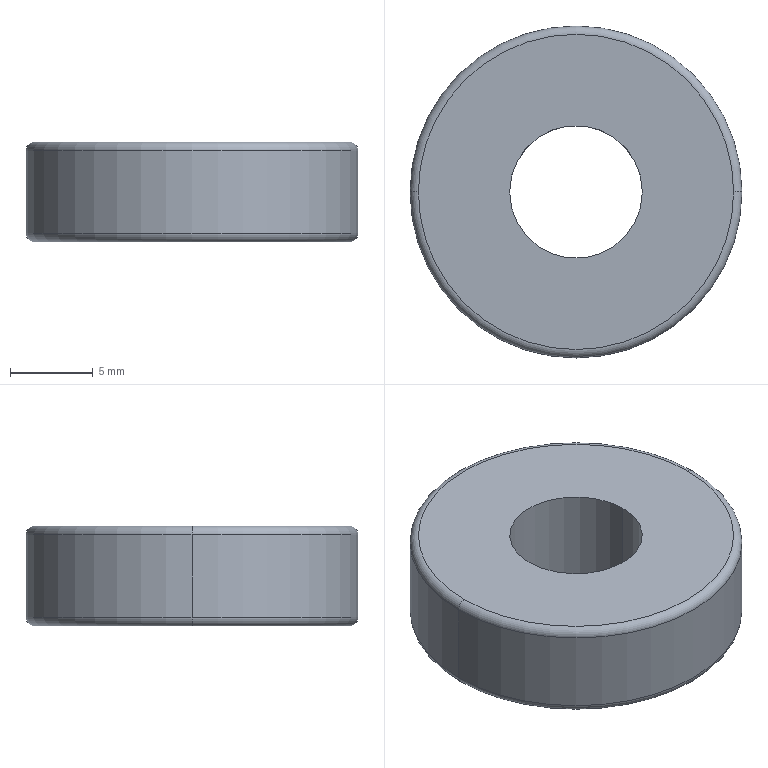Part | SolidWorks | features MirrorStock 1 | 1 solid | 10 faces | box 20 x 20 x 6 mm | volume 1577 mm3 | torus 4 | cylinder 4 | plane 2 | commonest cylinder face diameters 8 x2 20 x2
STEP:
#1=CARTESIAN_POINT('',(10.,0.,-5.5));
#2=VERTEX_POINT('',#1);
#3=CARTESIAN_POINT('',(-10.,0.,-5.5));
#4=VERTEX_POINT('',#3);
#5=CARTESIAN_POINT('',(0.,0.,-5.5));
#6=DIRECTION('',(0.,0.,-1.));
#7=DIRECTION('',(1.,0.,0.));
#8=AXIS2_PLACEMENT_3D('',#5,#6,#7);
#9=CIRCLE('',#8,10.);
#10=EDGE_CURVE('',#2,#4,#9,.T.);
#11=ORIENTED_EDGE('',*,*,#10,.T.);
#12=CARTESIAN_POINT('',(-9.5,0.,-6.));
#13=VERTEX_POINT('',#12);
#14=CARTESIAN_POINT('',(-9.5,0.,-5.5));
#15=DIRECTION('',(0.,-1.,0.));
#16=DIRECTION('',(1.,0.,0.));
#17=AXIS2_PLACEMENT_3D('',#14,#15,#16);
#18=CIRCLE('',#17,0.5);
#19=EDGE_CURVE('',#4,#13,#18,.T.);
#20=ORIENTED_EDGE('',*,*,#19,.T.);
#21=CARTESIAN_POINT('',(9.5,0.,-6.));
#22=VERTEX_POINT('',#21);
#23=CARTESIAN_POINT('',(0.,0.,-6.));
#24=DIRECTION('',(0.,0.,1.));
#25=DIRECTION('',(1.,0.,0.));
#26=AXIS2_PLACEMENT_3D('',#23,#24,#25);
#27=CIRCLE('',#26,9.5);
#28=EDGE_CURVE('',#13,#22,#27,.T.);
#29=ORIENTED_EDGE('',*,*,#28,.T.);
#30=CARTESIAN_POINT('',(9.5,0.,-5.5));
#31=DIRECTION('',(0.,1.,0.));
#32=DIRECTION('',(0.,0.,1.));
#33=AXIS2_PLACEMENT_3D('',#30,#31,#32);
#34=CIRCLE('',#33,0.5);
#35=EDGE_CURVE('',#2,#22,#34,.T.);
#36=ORIENTED_EDGE('',*,*,#35,.F.);
#37=EDGE_LOOP('',(#11,#20,#29,#36));
#38=FACE_OUTER_BOUND('',#37,.T.);
#39=CARTESIAN_POINT('',(0.,0.,-5.5));
#40=DIRECTION('',(0.,0.,-1.));
#41=DIRECTION('',(1.,0.,0.));
#42=AXIS2_PLACEMENT_3D('',#39,#40,#41);
#43=TOROIDAL_SURFACE('',#42,9.5,0.5);
#44=ADVANCED_FACE('',(#38),#43,.T.);
#45=CARTESIAN_POINT('',(9.5,0.,0.));
#46=VERTEX_POINT('',#45);
#47=CARTESIAN_POINT('',(-9.5,0.,0.));
#48=VERTEX_POINT('',#47);
#49=CARTESIAN_POINT('',(0.,0.,0.));
#50=DIRECTION('',(0.,0.,-1.));
#51=DIRECTION('',(1.,0.,0.));
#52=AXIS2_PLACEMENT_3D('',#49,#50,#51);
#53=CIRCLE('',#52,9.5);
#54=EDGE_CURVE('',#46,#48,#53,.T.);
#55=ORIENTED_EDGE('',*,*,#54,.T.);
#56=CARTESIAN_POINT('',(-10.,0.,-0.5));
#57=VERTEX_POINT('',#56);
#58=CARTESIAN_POINT('',(-9.5,0.,-0.5));
#59=DIRECTION('',(0.,-1.,0.));
#60=DIRECTION('',(1.,0.,0.));
#61=AXIS2_PLACEMENT_3D('',#58,#59,#60);
#62=CIRCLE('',#61,0.5);
#63=EDGE_CURVE('',#48,#57,#62,.T.);
#64=ORIENTED_EDGE('',*,*,#63,.T.);
#65=CARTESIAN_POINT('',(10.,0.,-0.5));
#66=VERTEX_POINT('',#65);
#67=CARTESIAN_POINT('',(0.,0.,-0.5));
#68=DIRECTION('',(0.,0.,1.));
#69=DIRECTION('',(1.,0.,0.));
#70=AXIS2_PLACEMENT_3D('',#67,#68,#69);
#71=CIRCLE('',#70,10.);
#72=EDGE_CURVE('',#57,#66,#71,.T.);
#73=ORIENTED_EDGE('',*,*,#72,.T.);
#74=CARTESIAN_POINT('',(9.5,0.,-0.5));
#75=DIRECTION('',(0.,1.,0.));
#76=DIRECTION('',(0.,0.,1.));
#77=AXIS2_PLACEMENT_3D('',#74,#75,#76);
#78=CIRCLE('',#77,0.5);
#79=EDGE_CURVE('',#46,#66,#78,.T.);
#80=ORIENTED_EDGE('',*,*,#79,.F.);
#81=EDGE_LOOP('',(#55,#64,#73,#80));
#82=FACE_OUTER_BOUND('',#81,.T.);
#83=CARTESIAN_POINT('',(0.,0.,-0.5));
#84=DIRECTION('',(0.,0.,-1.));
#85=DIRECTION('',(1.,0.,0.));
#86=AXIS2_PLACEMENT_3D('',#83,#84,#85);
#87=TOROIDAL_SURFACE('',#86,9.5,0.5);
#88=ADVANCED_FACE('',(#82),#87,.T.);
#89=CARTESIAN_POINT('',(4.,0.,-6.));
#90=VERTEX_POINT('',#89);
#91=CARTESIAN_POINT('',(-4.,0.,-6.));
#92=VERTEX_POINT('',#91);
#93=CARTESIAN_POINT('',(0.,0.,-6.));
#94=DIRECTION('',(0.,0.,1.));
#95=DIRECTION('',(1.,0.,0.));
#96=AXIS2_PLACEMENT_3D('',#93,#94,#95);
#97=CIRCLE('',#96,4.);
#98=EDGE_CURVE('',#90,#92,#97,.T.);
#99=ORIENTED_EDGE('',*,*,#98,.F.);
#100=CARTESIAN_POINT('',(4.,0.,0.));
#101=VERTEX_POINT('',#100);
#102=CARTESIAN_POINT('',(4.,0.,-6.));
#103=DIRECTION('',(0.,0.,1.));
#104=VECTOR('',#103,1000.);
#105=LINE('',#102,#104);
#106=EDGE_CURVE('',#90,#101,#105,.T.);
#107=ORIENTED_EDGE('',*,*,#106,.T.);
#108=CARTESIAN_POINT('',(-4.,0.,0.));
#109=VERTEX_POINT('',#108);
#110=CARTESIAN_POINT('',(0.,0.,0.));
#111=DIRECTION('',(0.,0.,1.));
#112=DIRECTION('',(1.,0.,0.));
#113=AXIS2_PLACEMENT_3D('',#110,#111,#112);
#114=CIRCLE('',#113,4.);
#115=EDGE_CURVE('',#101,#109,#114,.T.);
#116=ORIENTED_EDGE('',*,*,#115,.T.);
#117=CARTESIAN_POINT('',(-4.,0.,-6.));
#118=DIRECTION('',(0.,0.,1.));
#119=VECTOR('',#118,1000.);
#120=LINE('',#117,#119);
#121=EDGE_CURVE('',#92,#109,#120,.T.);
#122=ORIENTED_EDGE('',*,*,#121,.F.);
#123=EDGE_LOOP('',(#99,#107,#116,#122));
#124=FACE_OUTER_BOUND('',#123,.T.);
#125=CARTESIAN_POINT('',(0.,0.,-6.));
#126=DIRECTION('',(0.,0.,1.));
#127=DIRECTION('',(-1.,0.,0.));
#128=AXIS2_PLACEMENT_3D('',#125,#126,#127);
#129=CYLINDRICAL_SURFACE('',#128,4.);
#130=ADVANCED_FACE('',(#124),#129,.F.);
#131=ORIENTED_EDGE('',*,*,#10,.F.);
#132=CARTESIAN_POINT('',(10.,0.,-6.));
#133=DIRECTION('',(0.,0.,1.));
#134=VECTOR('',#133,1000.);
#135=LINE('',#132,#134);
#136=EDGE_CURVE('',#2,#66,#135,.T.);
#137=ORIENTED_EDGE('',*,*,#136,.T.);
#138=ORIENTED_EDGE('',*,*,#72,.F.);
#139=CARTESIAN_POINT('',(-10.,0.,-6.));
#140=DIRECTION('',(0.,0.,1.));
#141=VECTOR('',#140,1000.);
#142=LINE('',#139,#141);
#143=EDGE_CURVE('',#4,#57,#142,.T.);
#144=ORIENTED_EDGE('',*,*,#143,.F.);
#145=EDGE_LOOP('',(#131,#137,#138,#144));
#146=FACE_OUTER_BOUND('',#145,.T.);
#147=CARTESIAN_POINT('',(0.,0.,-6.));
#148=DIRECTION('',(0.,0.,1.));
#149=DIRECTION('',(-1.,0.,0.));
#150=AXIS2_PLACEMENT_3D('',#147,#148,#149);
#151=CYLINDRICAL_SURFACE('',#150,10.);
#152=ADVANCED_FACE('',(#146),#151,.T.);
#153=CARTESIAN_POINT('',(0.,0.,-6.));
#154=DIRECTION('',(0.,0.,1.));
#155=DIRECTION('',(1.,0.,0.));
#156=AXIS2_PLACEMENT_3D('',#153,#154,#155);
#157=CIRCLE('',#156,9.5);
#158=EDGE_CURVE('',#22,#13,#157,.T.);
#159=ORIENTED_EDGE('',*,*,#158,.F.);
#160=ORIENTED_EDGE('',*,*,#28,.F.);
#161=EDGE_LOOP('',(#159,#160));
#162=FACE_OUTER_BOUND('',#161,.T.);
#163=CARTESIAN_POINT('',(0.,0.,-6.));
#164=DIRECTION('',(0.,0.,1.));
#165=DIRECTION('',(1.,0.,0.));
#166=AXIS2_PLACEMENT_3D('',#163,#164,#165);
#167=CIRCLE('',#166,4.);
#168=EDGE_CURVE('',#92,#90,#167,.T.);
#169=ORIENTED_EDGE('',*,*,#168,.T.);
#170=ORIENTED_EDGE('',*,*,#98,.T.);
#171=EDGE_LOOP('',(#169,#170));
#172=FACE_BOUND('',#171,.T.);
#173=CARTESIAN_POINT('',(0.,0.,-6.));
#174=DIRECTION('',(0.,0.,-1.));
#175=DIRECTION('',(1.,0.,0.));
#176=AXIS2_PLACEMENT_3D('',#173,#174,#175);
#177=PLANE('',#176);
#178=ADVANCED_FACE('',(#162,#172),#177,.T.);
#179=ORIENTED_EDGE('',*,*,#54,.F.);
#180=CARTESIAN_POINT('',(0.,0.,0.));
#181=DIRECTION('',(0.,0.,-1.));
#182=DIRECTION('',(1.,0.,0.));
#183=AXIS2_PLACEMENT_3D('',#180,#181,#182);
#184=CIRCLE('',#183,9.5);
#185=EDGE_CURVE('',#48,#46,#184,.T.);
#186=ORIENTED_EDGE('',*,*,#185,.F.);
#187=EDGE_LOOP('',(#179,#186));
#188=FACE_OUTER_BOUND('',#187,.T.);
#189=CARTESIAN_POINT('',(0.,0.,0.));
#190=DIRECTION('',(0.,0.,1.));
#191=DIRECTION('',(1.,0.,0.));
#192=AXIS2_PLACEMENT_3D('',#189,#190,#191);
#193=CIRCLE('',#192,4.);
#194=EDGE_CURVE('',#109,#101,#193,.T.);
#195=ORIENTED_EDGE('',*,*,#194,.F.);
#196=ORIENTED_EDGE('',*,*,#115,.F.);
#197=EDGE_LOOP('',(#195,#196));
#198=FACE_BOUND('',#197,.T.);
#199=CARTESIAN_POINT('',(0.,0.,0.));
#200=DIRECTION('',(0.,0.,-1.));
#201=DIRECTION('',(1.,0.,0.));
#202=AXIS2_PLACEMENT_3D('',#199,#200,#201);
#203=PLANE('',#202);
#204=ADVANCED_FACE('',(#188,#198),#203,.F.);
#205=ORIENTED_EDGE('',*,*,#136,.F.);
#206=CARTESIAN_POINT('',(0.,0.,-5.5));
#207=DIRECTION('',(0.,0.,-1.));
#208=DIRECTION('',(1.,0.,0.));
#209=AXIS2_PLACEMENT_3D('',#206,#207,#208);
#210=CIRCLE('',#209,10.);
#211=EDGE_CURVE('',#4,#2,#210,.T.);
#212=ORIENTED_EDGE('',*,*,#211,.F.);
#213=ORIENTED_EDGE('',*,*,#143,.T.);
#214=CARTESIAN_POINT('',(0.,0.,-0.5));
#215=DIRECTION('',(0.,0.,1.));
#216=DIRECTION('',(1.,0.,0.));
#217=AXIS2_PLACEMENT_3D('',#214,#215,#216);
#218=CIRCLE('',#217,10.);
#219=EDGE_CURVE('',#66,#57,#218,.T.);
#220=ORIENTED_EDGE('',*,*,#219,.F.);
#221=EDGE_LOOP('',(#205,#212,#213,#220));
#222=FACE_OUTER_BOUND('',#221,.T.);
#223=CARTESIAN_POINT('',(0.,0.,-6.));
#224=DIRECTION('',(0.,0.,1.));
#225=DIRECTION('',(-1.,0.,0.));
#226=AXIS2_PLACEMENT_3D('',#223,#224,#225);
#227=CYLINDRICAL_SURFACE('',#226,10.);
#228=ADVANCED_FACE('',(#222),#227,.T.);
#229=ORIENTED_EDGE('',*,*,#106,.F.);
#230=ORIENTED_EDGE('',*,*,#168,.F.);
#231=ORIENTED_EDGE('',*,*,#121,.T.);
#232=ORIENTED_EDGE('',*,*,#194,.T.);
#233=EDGE_LOOP('',(#229,#230,#231,#232));
#234=FACE_OUTER_BOUND('',#233,.T.);
#235=CARTESIAN_POINT('',(0.,0.,-6.));
#236=DIRECTION('',(0.,0.,1.));
#237=DIRECTION('',(-1.,0.,0.));
#238=AXIS2_PLACEMENT_3D('',#235,#236,#237);
#239=CYLINDRICAL_SURFACE('',#238,4.);
#240=ADVANCED_FACE('',(#234),#239,.F.);
#241=ORIENTED_EDGE('',*,*,#63,.F.);
#242=ORIENTED_EDGE('',*,*,#185,.T.);
#243=ORIENTED_EDGE('',*,*,#79,.T.);
#244=ORIENTED_EDGE('',*,*,#219,.T.);
#245=EDGE_LOOP('',(#241,#242,#243,#244));
#246=FACE_OUTER_BOUND('',#245,.T.);
#247=CARTESIAN_POINT('',(0.,0.,-0.5));
#248=DIRECTION('',(0.,0.,-1.));
#249=DIRECTION('',(1.,0.,0.));
#250=AXIS2_PLACEMENT_3D('',#247,#248,#249);
#251=TOROIDAL_SURFACE('',#250,9.5,0.5);
#252=ADVANCED_FACE('',(#246),#251,.T.);
#253=ORIENTED_EDGE('',*,*,#19,.F.);
#254=ORIENTED_EDGE('',*,*,#211,.T.);
#255=ORIENTED_EDGE('',*,*,#35,.T.);
#256=ORIENTED_EDGE('',*,*,#158,.T.);
#257=EDGE_LOOP('',(#253,#254,#255,#256));
#258=FACE_OUTER_BOUND('',#257,.T.);
#259=CARTESIAN_POINT('',(0.,0.,-5.5));
#260=DIRECTION('',(0.,0.,-1.));
#261=DIRECTION('',(1.,0.,0.));
#262=AXIS2_PLACEMENT_3D('',#259,#260,#261);
#263=TOROIDAL_SURFACE('',#262,9.5,0.5);
#264=ADVANCED_FACE('',(#258),#263,.T.);
#265=CLOSED_SHELL('',(#44,#88,#130,#152,#178,#204,#228,#240,#252,#264));
#266=MANIFOLD_SOLID_BREP('',#265);
#267=CARTESIAN_POINT('',(0.,0.,0.));
#268=DIRECTION('',(0.,0.,1.));
#269=DIRECTION('',(1.,0.,0.));
#270=AXIS2_PLACEMENT_3D('',#267,#268,#269);
#271=(LENGTH_UNIT()NAMED_UNIT(*)SI_UNIT(.MILLI.,.METRE.));
#272=UNCERTAINTY_MEASURE_WITH_UNIT(LENGTH_MEASURE(0.00001),#271,'','');
#273=(NAMED_UNIT(*)PLANE_ANGLE_UNIT()SI_UNIT($,.RADIAN.));
#274=(NAMED_UNIT(*)SI_UNIT($,.STERADIAN.)SOLID_ANGLE_UNIT());
#275=(GEOMETRIC_REPRESENTATION_CONTEXT(3)GLOBAL_UNCERTAINTY_ASSIGNED_CONTEXT((#272))GLOBAL_UNIT_ASSIGNED_CONTEXT((#271,#273,#274))REPRESENTATION_CONTEXT('',''));
#276=ADVANCED_BREP_SHAPE_REPRESENTATION('',(#266,#270),#275);